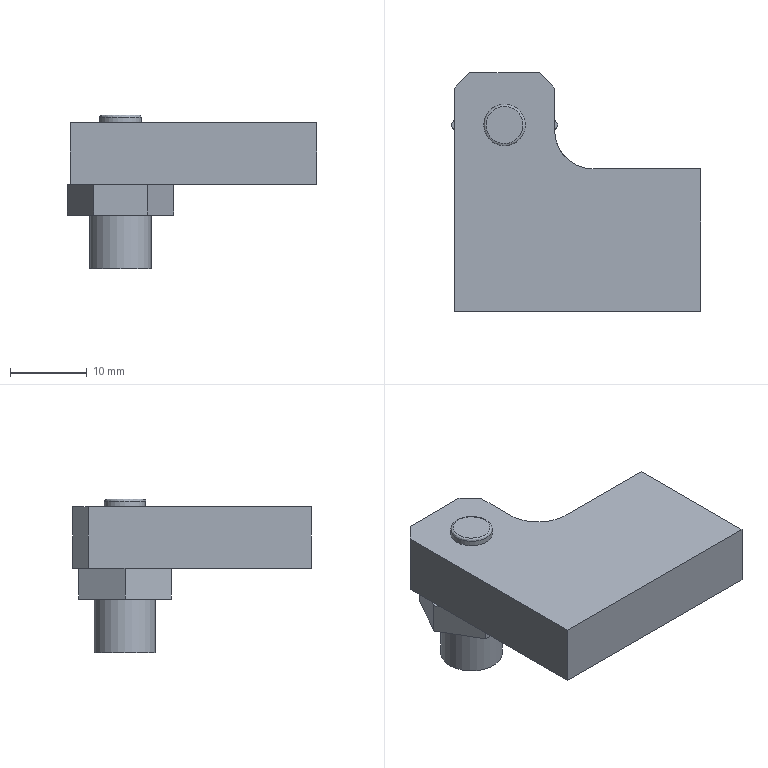Part | NX | 1 solid | 81 faces | box 32.429 x 31 x 20 mm | volume 6634 mm3 | plane 65 | cylinder 11 | cone 4 | spline 1 | commonest cylinder face diameters 7 x4 7.5 x4 5.4 x1 8 x1 10 x1